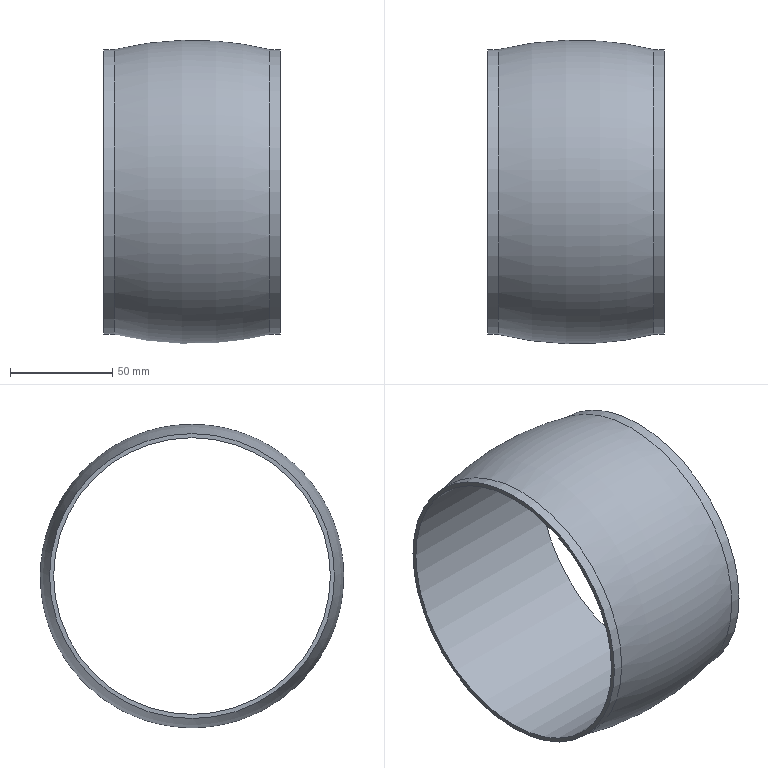Part | NX | features BREP 1 | 1 solid | 6 faces | box 86 x 148.156 x 148.156 mm | volume 178291 mm3 | cylinder 3 | plane 2 | torus 1 | commonest cylinder face diameters 139 x2 135 x1
STEP:
#1=CARTESIAN_POINT('',(0.,0.,69.5));
#2=VERTEX_POINT('',#1);
#3=CARTESIAN_POINT('',(0.,0.,0.));
#4=DIRECTION('',(-1.,0.,0.));
#5=DIRECTION('',(0.,0.,1.));
#6=AXIS2_PLACEMENT_3D('',#3,#4,#5);
#7=CIRCLE('',#6,69.5);
#8=EDGE_CURVE('',#2,#2,#7,.T.);
#9=ORIENTED_EDGE('',*,*,#8,.F.);
#10=EDGE_LOOP('',(#9));
#11=FACE_BOUND('',#10,.T.);
#12=CARTESIAN_POINT('',(5.,0.,69.5));
#13=VERTEX_POINT('',#12);
#14=CARTESIAN_POINT('',(5.,0.,0.));
#15=DIRECTION('',(-1.,0.,0.));
#16=DIRECTION('',(0.,0.,1.));
#17=AXIS2_PLACEMENT_3D('',#14,#15,#16);
#18=CIRCLE('',#17,69.5);
#19=EDGE_CURVE('',#13,#13,#18,.T.);
#20=ORIENTED_EDGE('',*,*,#19,.T.);
#21=EDGE_LOOP('',(#20));
#22=FACE_BOUND('',#21,.T.);
#23=CARTESIAN_POINT('',(0.,0.,0.));
#24=DIRECTION('',(-1.,0.,0.));
#25=DIRECTION('',(0.,0.,1.));
#26=AXIS2_PLACEMENT_3D('',#23,#24,#25);
#27=CYLINDRICAL_SURFACE('',#26,69.5);
#28=ADVANCED_FACE('',(#11,#22),#27,.T.);
#29=ORIENTED_EDGE('',*,*,#19,.F.);
#30=EDGE_LOOP('',(#29));
#31=FACE_BOUND('',#30,.T.);
#32=CARTESIAN_POINT('',(81.,0.,69.5));
#33=VERTEX_POINT('',#32);
#34=CARTESIAN_POINT('',(81.,0.,0.));
#35=DIRECTION('',(-1.,0.,0.));
#36=DIRECTION('',(0.,0.,1.));
#37=AXIS2_PLACEMENT_3D('',#34,#35,#36);
#38=CIRCLE('',#37,69.5);
#39=EDGE_CURVE('',#33,#33,#38,.T.);
#40=ORIENTED_EDGE('',*,*,#39,.T.);
#41=EDGE_LOOP('',(#40));
#42=FACE_BOUND('',#41,.T.);
#43=CARTESIAN_POINT('',(43.,0.,0.));
#44=DIRECTION('',(-1.,0.,0.));
#45=DIRECTION('',(0.,0.,1.));
#46=AXIS2_PLACEMENT_3D('',#43,#44,#45);
#47=DEGENERATE_TOROIDAL_SURFACE('',#46,85.922,160.,.F.);
#48=ADVANCED_FACE('',(#31,#42),#47,.F.);
#49=ORIENTED_EDGE('',*,*,#39,.F.);
#50=EDGE_LOOP('',(#49));
#51=FACE_BOUND('',#50,.T.);
#52=CARTESIAN_POINT('',(86.,0.,69.5));
#53=VERTEX_POINT('',#52);
#54=CARTESIAN_POINT('',(86.,0.,0.));
#55=DIRECTION('',(-1.,0.,0.));
#56=DIRECTION('',(0.,0.,1.));
#57=AXIS2_PLACEMENT_3D('',#54,#55,#56);
#58=CIRCLE('',#57,69.5);
#59=EDGE_CURVE('',#53,#53,#58,.T.);
#60=ORIENTED_EDGE('',*,*,#59,.T.);
#61=EDGE_LOOP('',(#60));
#62=FACE_BOUND('',#61,.T.);
#63=CARTESIAN_POINT('',(0.,0.,0.));
#64=DIRECTION('',(-1.,0.,0.));
#65=DIRECTION('',(0.,0.,1.));
#66=AXIS2_PLACEMENT_3D('',#63,#64,#65);
#67=CYLINDRICAL_SURFACE('',#66,69.5);
#68=ADVANCED_FACE('',(#51,#62),#67,.T.);
#69=CARTESIAN_POINT('',(0.,0.,67.5));
#70=VERTEX_POINT('',#69);
#71=CARTESIAN_POINT('',(0.,0.,0.));
#72=DIRECTION('',(-1.,0.,0.));
#73=DIRECTION('',(0.,0.,1.));
#74=AXIS2_PLACEMENT_3D('',#71,#72,#73);
#75=CIRCLE('',#74,67.5);
#76=EDGE_CURVE('',#70,#70,#75,.T.);
#77=ORIENTED_EDGE('',*,*,#76,.T.);
#78=EDGE_LOOP('',(#77));
#79=FACE_BOUND('',#78,.T.);
#80=CARTESIAN_POINT('',(86.,0.,67.5));
#81=VERTEX_POINT('',#80);
#82=CARTESIAN_POINT('',(86.,0.,0.));
#83=DIRECTION('',(-1.,0.,0.));
#84=DIRECTION('',(0.,0.,1.));
#85=AXIS2_PLACEMENT_3D('',#82,#83,#84);
#86=CIRCLE('',#85,67.5);
#87=EDGE_CURVE('',#81,#81,#86,.T.);
#88=ORIENTED_EDGE('',*,*,#87,.F.);
#89=EDGE_LOOP('',(#88));
#90=FACE_BOUND('',#89,.T.);
#91=CARTESIAN_POINT('',(0.,0.,0.));
#92=DIRECTION('',(-1.,0.,0.));
#93=DIRECTION('',(0.,0.,1.));
#94=AXIS2_PLACEMENT_3D('',#91,#92,#93);
#95=CYLINDRICAL_SURFACE('',#94,67.5);
#96=ADVANCED_FACE('',(#79,#90),#95,.F.);
#97=ORIENTED_EDGE('',*,*,#76,.F.);
#98=EDGE_LOOP('',(#97));
#99=FACE_BOUND('',#98,.T.);
#100=ORIENTED_EDGE('',*,*,#8,.T.);
#101=EDGE_LOOP('',(#100));
#102=FACE_BOUND('',#101,.T.);
#103=CARTESIAN_POINT('',(0.,67.5,0.));
#104=DIRECTION('',(1.,0.,0.));
#105=DIRECTION('',(0.,0.,-1.));
#106=AXIS2_PLACEMENT_3D('',#103,#104,#105);
#107=PLANE('',#106);
#108=ADVANCED_FACE('',(#99,#102),#107,.F.);
#109=ORIENTED_EDGE('',*,*,#59,.F.);
#110=EDGE_LOOP('',(#109));
#111=FACE_BOUND('',#110,.T.);
#112=ORIENTED_EDGE('',*,*,#87,.T.);
#113=EDGE_LOOP('',(#112));
#114=FACE_BOUND('',#113,.T.);
#115=CARTESIAN_POINT('',(86.,69.5,0.));
#116=DIRECTION('',(-1.,0.,0.));
#117=DIRECTION('',(0.,0.,1.));
#118=AXIS2_PLACEMENT_3D('',#115,#116,#117);
#119=PLANE('',#118);
#120=ADVANCED_FACE('',(#111,#114),#119,.F.);
#121=CLOSED_SHELL('',(#28,#48,#68,#96,#108,#120));
#122=MANIFOLD_SOLID_BREP('',#121);
#123=(LENGTH_UNIT()NAMED_UNIT(*)SI_UNIT(.MILLI.,.METRE.));
#124=UNCERTAINTY_MEASURE_WITH_UNIT(LENGTH_MEASURE(0.00001),#123,'','');
#125=(NAMED_UNIT(*)PLANE_ANGLE_UNIT()SI_UNIT($,.RADIAN.));
#126=(NAMED_UNIT(*)SI_UNIT($,.STERADIAN.)SOLID_ANGLE_UNIT());
#127=(GEOMETRIC_REPRESENTATION_CONTEXT(3)GLOBAL_UNCERTAINTY_ASSIGNED_CONTEXT((#124))GLOBAL_UNIT_ASSIGNED_CONTEXT((#123,#125,#126))REPRESENTATION_CONTEXT('',''));
#128=ADVANCED_BREP_SHAPE_REPRESENTATION('',(#122),#127);